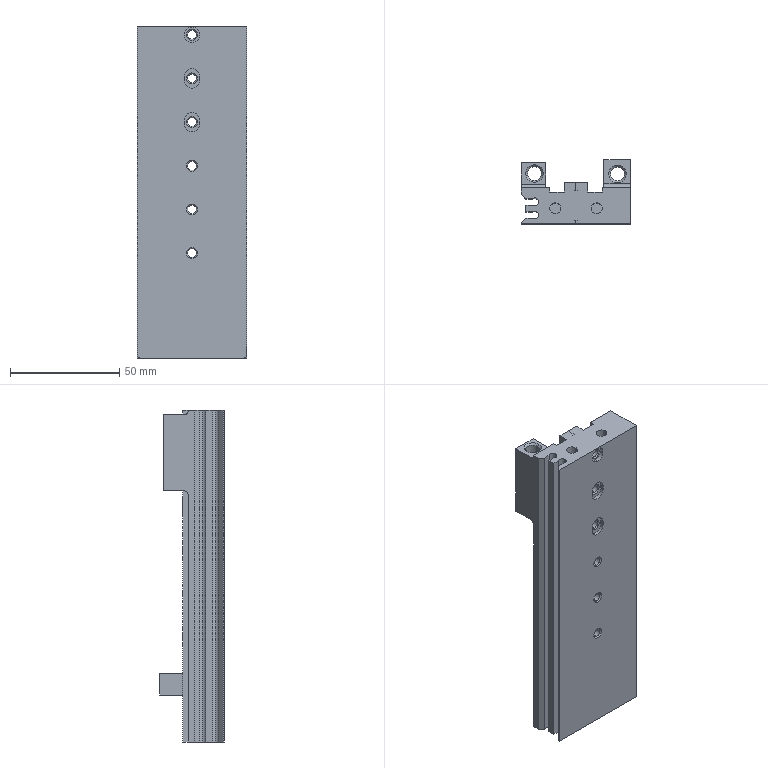Part | STEP file | 1 solid | 160 faces | box 50 x 29.5 x 152 mm | volume 104448 mm3 | cylinder 66 | plane 51 | cone 43 | commonest cylinder face diameters 4 x22 8 x10 7 x8 2.4 x6 3.6 x4 5 x4